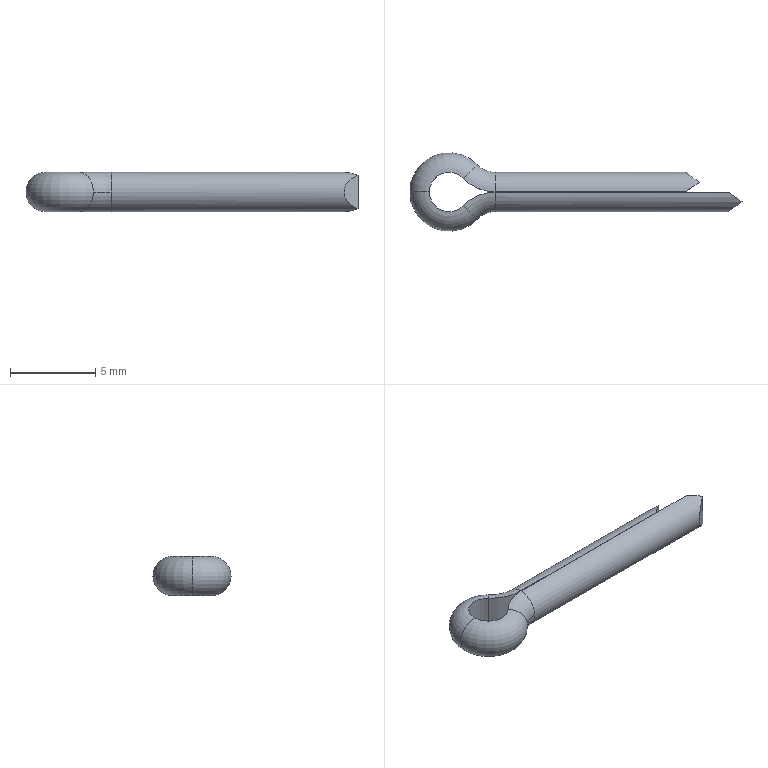Part | SolidWorks | features ICE 1, Sweep 1 | 1 solid | 17 faces | box 19.5 x 4.6 x 2.3 mm | volume 75.866 mm3 | torus 6 | plane 6 | cylinder 5 | commonest cylinder face diameters 2.3 x2 5.169 x2 2.32 x1
STEP:
#1=CARTESIAN_POINT('',(2.7,0.01,1.15));
#2=VERTEX_POINT('',#1);
#3=CARTESIAN_POINT('',(2.7,1.15,0.));
#4=VERTEX_POINT('',#3);
#5=CARTESIAN_POINT('',(2.7,0.,0.));
#6=DIRECTION('',(-1.,0.,0.));
#7=DIRECTION('',(0.,0.,1.));
#8=AXIS2_PLACEMENT_3D('',#5,#6,#7);
#9=CIRCLE('',#8,1.15);
#10=EDGE_CURVE('',#2,#4,#9,.T.);
#11=ORIENTED_EDGE('',*,*,#10,.T.);
#12=CARTESIAN_POINT('',(1.658,1.594,0.));
#13=VERTEX_POINT('',#12);
#14=CARTESIAN_POINT('',(2.7,2.595,0.));
#15=DIRECTION('',(0.,0.,-1.));
#16=DIRECTION('',(-1.,0.,0.));
#17=AXIS2_PLACEMENT_3D('',#14,#15,#16);
#18=CIRCLE('',#17,1.445);
#19=EDGE_CURVE('',#4,#13,#18,.T.);
#20=ORIENTED_EDGE('',*,*,#19,.T.);
#21=CARTESIAN_POINT('',(0.8364,0.8038,1.15));
#22=VERTEX_POINT('',#21);
#23=CARTESIAN_POINT('',(0.8292,0.7968,0.));
#24=DIRECTION('',(-0.6929,0.721,0.));
#25=DIRECTION('',(0.,0.,1.));
#26=AXIS2_PLACEMENT_3D('',#23,#24,#25);
#27=CIRCLE('',#26,1.15);
#28=EDGE_CURVE('',#22,#13,#27,.T.);
#29=ORIENTED_EDGE('',*,*,#28,.F.);
#30=CARTESIAN_POINT('',(2.7,2.595,1.15));
#31=DIRECTION('',(0.,0.,-1.));
#32=DIRECTION('',(-1.,0.,0.));
#33=AXIS2_PLACEMENT_3D('',#30,#31,#32);
#34=CIRCLE('',#33,2.585);
#35=EDGE_CURVE('',#2,#22,#34,.T.);
#36=ORIENTED_EDGE('',*,*,#35,.F.);
#37=EDGE_LOOP('',(#11,#20,#29,#36));
#38=FACE_OUTER_BOUND('',#37,.T.);
#39=CARTESIAN_POINT('',(2.7,2.595,0.));
#40=DIRECTION('',(0.,0.,-1.));
#41=DIRECTION('',(-1.,0.,0.));
#42=AXIS2_PLACEMENT_3D('',#39,#40,#41);
#43=TOROIDAL_SURFACE('',#42,2.595,1.15);
#44=ADVANCED_FACE('',(#38),#43,.T.);
#45=CARTESIAN_POINT('',(0.8364,-0.8038,1.15));
#46=VERTEX_POINT('',#45);
#47=CARTESIAN_POINT('',(1.658,-1.594,0.));
#48=VERTEX_POINT('',#47);
#49=CARTESIAN_POINT('',(0.8292,-0.7968,0.));
#50=DIRECTION('',(0.6929,0.721,0.));
#51=DIRECTION('',(0.,0.,1.));
#52=AXIS2_PLACEMENT_3D('',#49,#50,#51);
#53=CIRCLE('',#52,1.15);
#54=EDGE_CURVE('',#46,#48,#53,.T.);
#55=ORIENTED_EDGE('',*,*,#54,.T.);
#56=CARTESIAN_POINT('',(2.7,-1.15,0.));
#57=VERTEX_POINT('',#56);
#58=CARTESIAN_POINT('',(2.7,-2.595,0.));
#59=DIRECTION('',(0.,0.,-1.));
#60=DIRECTION('',(-1.,0.,0.));
#61=AXIS2_PLACEMENT_3D('',#58,#59,#60);
#62=CIRCLE('',#61,1.445);
#63=EDGE_CURVE('',#48,#57,#62,.T.);
#64=ORIENTED_EDGE('',*,*,#63,.T.);
#65=CARTESIAN_POINT('',(2.7,-0.01,1.15));
#66=VERTEX_POINT('',#65);
#67=CARTESIAN_POINT('',(2.7,0.,0.));
#68=DIRECTION('',(1.,0.,0.));
#69=DIRECTION('',(0.,0.,1.));
#70=AXIS2_PLACEMENT_3D('',#67,#68,#69);
#71=CIRCLE('',#70,1.15);
#72=EDGE_CURVE('',#66,#57,#71,.T.);
#73=ORIENTED_EDGE('',*,*,#72,.F.);
#74=CARTESIAN_POINT('',(2.7,-2.595,1.15));
#75=DIRECTION('',(0.,0.,-1.));
#76=DIRECTION('',(-1.,0.,0.));
#77=AXIS2_PLACEMENT_3D('',#74,#75,#76);
#78=CIRCLE('',#77,2.585);
#79=EDGE_CURVE('',#46,#66,#78,.T.);
#80=ORIENTED_EDGE('',*,*,#79,.F.);
#81=EDGE_LOOP('',(#55,#64,#73,#80));
#82=FACE_OUTER_BOUND('',#81,.T.);
#83=CARTESIAN_POINT('',(2.7,-2.595,0.));
#84=DIRECTION('',(0.,0.,-1.));
#85=DIRECTION('',(-1.,0.,0.));
#86=AXIS2_PLACEMENT_3D('',#83,#84,#85);
#87=TOROIDAL_SURFACE('',#86,2.595,1.15);
#88=ADVANCED_FACE('',(#82),#87,.T.);
#89=CARTESIAN_POINT('',(0.8364,0.8038,-1.15));
#90=VERTEX_POINT('',#89);
#91=CARTESIAN_POINT('',(-1.16,0.,-1.15));
#92=VERTEX_POINT('',#91);
#93=CARTESIAN_POINT('',(0.,0.,-1.15));
#94=DIRECTION('',(0.,0.,1.));
#95=DIRECTION('',(1.,0.,0.));
#96=AXIS2_PLACEMENT_3D('',#93,#94,#95);
#97=CIRCLE('',#96,1.16);
#98=EDGE_CURVE('',#90,#92,#97,.T.);
#99=ORIENTED_EDGE('',*,*,#98,.T.);
#100=CARTESIAN_POINT('',(-1.16,0.,1.15));
#101=VERTEX_POINT('',#100);
#102=CARTESIAN_POINT('',(-1.15,0.,0.));
#103=DIRECTION('',(0.,1.,0.));
#104=DIRECTION('',(-1.,0.,0.));
#105=AXIS2_PLACEMENT_3D('',#102,#103,#104);
#106=CIRCLE('',#105,1.15);
#107=EDGE_CURVE('',#92,#101,#106,.T.);
#108=ORIENTED_EDGE('',*,*,#107,.T.);
#109=CARTESIAN_POINT('',(0.,0.,1.15));
#110=DIRECTION('',(0.,0.,1.));
#111=DIRECTION('',(1.,0.,0.));
#112=AXIS2_PLACEMENT_3D('',#109,#110,#111);
#113=CIRCLE('',#112,1.16);
#114=EDGE_CURVE('',#22,#101,#113,.T.);
#115=ORIENTED_EDGE('',*,*,#114,.F.);
#116=ORIENTED_EDGE('',*,*,#28,.T.);
#117=CARTESIAN_POINT('',(0.8292,0.7968,0.));
#118=DIRECTION('',(-0.6929,0.721,0.));
#119=DIRECTION('',(0.,0.,1.));
#120=AXIS2_PLACEMENT_3D('',#117,#118,#119);
#121=CIRCLE('',#120,1.15);
#122=EDGE_CURVE('',#13,#90,#121,.T.);
#123=ORIENTED_EDGE('',*,*,#122,.T.);
#124=EDGE_LOOP('',(#99,#108,#115,#116,#123));
#125=FACE_OUTER_BOUND('',#124,.T.);
#126=CARTESIAN_POINT('',(0.,0.,0.));
#127=DIRECTION('',(0.,0.,1.));
#128=DIRECTION('',(1.,0.,0.));
#129=AXIS2_PLACEMENT_3D('',#126,#127,#128);
#130=TOROIDAL_SURFACE('',#129,1.15,1.15);
#131=ADVANCED_FACE('',(#125),#130,.T.);
#132=CARTESIAN_POINT('',(17.2,-0.58,-0.993));
#133=VERTEX_POINT('',#132);
#134=CARTESIAN_POINT('',(16.396,-0.01,-1.15));
#135=VERTEX_POINT('',#134);
#136=CARTESIAN_POINT('',(17.2,-0.58,-0.993));
#137=CARTESIAN_POINT('',(16.955,-0.4059,-1.095));
#138=CARTESIAN_POINT('',(16.681,-0.2116,-1.148));
#139=CARTESIAN_POINT('',(16.396,-0.01,-1.15));
#140=(BOUNDED_CURVE()B_SPLINE_CURVE(3,(#136,#137,#138,#139),.UNSPECIFIED.,.F.,.F.)B_SPLINE_CURVE_WITH_KNOTS((4,4),(1.042,1.562),.UNSPECIFIED.)CURVE()GEOMETRIC_REPRESENTATION_ITEM()RATIONAL_B_SPLINE_CURVE((1.,0.9776,0.9776,1.))REPRESENTATION_ITEM(''));
#141=EDGE_CURVE('',#133,#135,#140,.T.);
#142=ORIENTED_EDGE('',*,*,#141,.F.);
#143=CARTESIAN_POINT('',(17.2,-0.58,0.993));
#144=VERTEX_POINT('',#143);
#145=CARTESIAN_POINT('',(17.2,-0.58,0.993));
#146=CARTESIAN_POINT('',(15.965,-1.434,0.4944));
#147=CARTESIAN_POINT('',(15.965,-1.434,-0.4944));
#148=CARTESIAN_POINT('',(17.2,-0.58,-0.993));
#149=(BOUNDED_CURVE()B_SPLINE_CURVE(3,(#145,#146,#147,#148),.UNSPECIFIED.,.F.,.F.)B_SPLINE_CURVE_WITH_KNOTS((4,4),(2.099,4.184),.UNSPECIFIED.)CURVE()GEOMETRIC_REPRESENTATION_ITEM()RATIONAL_B_SPLINE_CURVE((1.,0.6696,0.6696,1.))REPRESENTATION_ITEM(''));
#150=EDGE_CURVE('',#144,#133,#149,.T.);
#151=ORIENTED_EDGE('',*,*,#150,.F.);
#152=CARTESIAN_POINT('',(16.396,-0.01,1.15));
#153=VERTEX_POINT('',#152);
#154=CARTESIAN_POINT('',(16.396,-0.01,1.15));
#155=CARTESIAN_POINT('',(16.681,-0.2116,1.148));
#156=CARTESIAN_POINT('',(16.955,-0.4059,1.095));
#157=CARTESIAN_POINT('',(17.2,-0.58,0.993));
#158=(BOUNDED_CURVE()B_SPLINE_CURVE(3,(#154,#155,#156,#157),.UNSPECIFIED.,.F.,.F.)B_SPLINE_CURVE_WITH_KNOTS((4,4),(4.721,5.241),.UNSPECIFIED.)CURVE()GEOMETRIC_REPRESENTATION_ITEM()RATIONAL_B_SPLINE_CURVE((1.,0.9776,0.9776,1.))REPRESENTATION_ITEM(''));
#159=EDGE_CURVE('',#153,#144,#158,.T.);
#160=ORIENTED_EDGE('',*,*,#159,.F.);
#161=CARTESIAN_POINT('',(2.7,-0.01,1.15));
#162=DIRECTION('',(1.,0.,0.));
#163=VECTOR('',#162,1000.);
#164=LINE('',#161,#163);
#165=EDGE_CURVE('',#66,#153,#164,.T.);
#166=ORIENTED_EDGE('',*,*,#165,.F.);
#167=ORIENTED_EDGE('',*,*,#72,.T.);
#168=CARTESIAN_POINT('',(2.7,-0.01,-1.15));
#169=VERTEX_POINT('',#168);
#170=CARTESIAN_POINT('',(2.7,0.,0.));
#171=DIRECTION('',(1.,0.,0.));
#172=DIRECTION('',(0.,0.,1.));
#173=AXIS2_PLACEMENT_3D('',#170,#171,#172);
#174=CIRCLE('',#173,1.15);
#175=EDGE_CURVE('',#57,#169,#174,.T.);
#176=ORIENTED_EDGE('',*,*,#175,.T.);
#177=CARTESIAN_POINT('',(2.7,-0.01,-1.15));
#178=DIRECTION('',(1.,0.,0.));
#179=VECTOR('',#178,1000.);
#180=LINE('',#177,#179);
#181=EDGE_CURVE('',#169,#135,#180,.T.);
#182=ORIENTED_EDGE('',*,*,#181,.T.);
#183=EDGE_LOOP('',(#142,#151,#160,#166,#167,#176,#182));
#184=FACE_OUTER_BOUND('',#183,.T.);
#185=CARTESIAN_POINT('',(2.7,0.,0.));
#186=DIRECTION('',(1.,0.,0.));
#187=DIRECTION('',(0.,1.,0.));
#188=AXIS2_PLACEMENT_3D('',#185,#186,#187);
#189=CYLINDRICAL_SURFACE('',#188,1.15);
#190=ADVANCED_FACE('',(#184),#189,.T.);
#191=CARTESIAN_POINT('',(16.396,-0.01,-1.15));
#192=DIRECTION('',(0.,0.,1.));
#193=VECTOR('',#192,1000.);
#194=LINE('',#191,#193);
#195=EDGE_CURVE('',#135,#153,#194,.T.);
#196=ORIENTED_EDGE('',*,*,#195,.F.);
#197=ORIENTED_EDGE('',*,*,#181,.F.);
#198=CARTESIAN_POINT('',(2.7,-0.01,-1.15));
#199=DIRECTION('',(0.,0.,1.));
#200=VECTOR('',#199,1000.);
#201=LINE('',#198,#200);
#202=EDGE_CURVE('',#169,#66,#201,.T.);
#203=ORIENTED_EDGE('',*,*,#202,.T.);
#204=ORIENTED_EDGE('',*,*,#165,.T.);
#205=EDGE_LOOP('',(#196,#197,#203,#204));
#206=FACE_OUTER_BOUND('',#205,.T.);
#207=CARTESIAN_POINT('',(2.7,-0.01,-1.15));
#208=DIRECTION('',(0.,1.,0.));
#209=DIRECTION('',(-1.,0.,0.));
#210=AXIS2_PLACEMENT_3D('',#207,#208,#209);
#211=PLANE('',#210);
#212=ADVANCED_FACE('',(#206),#211,.T.);
#213=CARTESIAN_POINT('',(0.8364,-0.8038,-1.15));
#214=VERTEX_POINT('',#213);
#215=CARTESIAN_POINT('',(0.8364,-0.8038,-1.15));
#216=DIRECTION('',(0.,0.,1.));
#217=VECTOR('',#216,1000.);
#218=LINE('',#215,#217);
#219=EDGE_CURVE('',#214,#46,#218,.T.);
#220=ORIENTED_EDGE('',*,*,#219,.T.);
#221=ORIENTED_EDGE('',*,*,#79,.T.);
#222=ORIENTED_EDGE('',*,*,#202,.F.);
#223=CARTESIAN_POINT('',(2.7,-2.595,-1.15));
#224=DIRECTION('',(0.,0.,-1.));
#225=DIRECTION('',(-1.,0.,0.));
#226=AXIS2_PLACEMENT_3D('',#223,#224,#225);
#227=CIRCLE('',#226,2.585);
#228=EDGE_CURVE('',#214,#169,#227,.T.);
#229=ORIENTED_EDGE('',*,*,#228,.F.);
#230=EDGE_LOOP('',(#220,#221,#222,#229));
#231=FACE_OUTER_BOUND('',#230,.T.);
#232=CARTESIAN_POINT('',(2.7,-2.595,0.));
#233=DIRECTION('',(0.,0.,-1.));
#234=DIRECTION('',(-1.,0.,0.));
#235=AXIS2_PLACEMENT_3D('',#232,#233,#234);
#236=CYLINDRICAL_SURFACE('',#235,2.585);
#237=ADVANCED_FACE('',(#231),#236,.T.);
#238=ORIENTED_EDGE('',*,*,#63,.F.);
#239=CARTESIAN_POINT('',(0.8292,-0.7968,0.));
#240=DIRECTION('',(0.6929,0.721,0.));
#241=DIRECTION('',(0.,0.,1.));
#242=AXIS2_PLACEMENT_3D('',#239,#240,#241);
#243=CIRCLE('',#242,1.15);
#244=EDGE_CURVE('',#48,#214,#243,.T.);
#245=ORIENTED_EDGE('',*,*,#244,.T.);
#246=ORIENTED_EDGE('',*,*,#228,.T.);
#247=ORIENTED_EDGE('',*,*,#175,.F.);
#248=EDGE_LOOP('',(#238,#245,#246,#247));
#249=FACE_OUTER_BOUND('',#248,.T.);
#250=CARTESIAN_POINT('',(2.7,-2.595,0.));
#251=DIRECTION('',(0.,0.,-1.));
#252=DIRECTION('',(-1.,0.,0.));
#253=AXIS2_PLACEMENT_3D('',#250,#251,#252);
#254=TOROIDAL_SURFACE('',#253,2.595,1.15);
#255=ADVANCED_FACE('',(#249),#254,.T.);
#256=CARTESIAN_POINT('',(0.8364,0.8038,-1.15));
#257=DIRECTION('',(0.,0.,1.));
#258=VECTOR('',#257,1000.);
#259=LINE('',#256,#258);
#260=EDGE_CURVE('',#90,#22,#259,.T.);
#261=ORIENTED_EDGE('',*,*,#260,.T.);
#262=ORIENTED_EDGE('',*,*,#114,.T.);
#263=CARTESIAN_POINT('',(0.,0.,1.15));
#264=DIRECTION('',(0.,0.,1.));
#265=DIRECTION('',(1.,0.,0.));
#266=AXIS2_PLACEMENT_3D('',#263,#264,#265);
#267=CIRCLE('',#266,1.16);
#268=EDGE_CURVE('',#101,#46,#267,.T.);
#269=ORIENTED_EDGE('',*,*,#268,.T.);
#270=ORIENTED_EDGE('',*,*,#219,.F.);
#271=CARTESIAN_POINT('',(0.,0.,-1.15));
#272=DIRECTION('',(0.,0.,1.));
#273=DIRECTION('',(1.,0.,0.));
#274=AXIS2_PLACEMENT_3D('',#271,#272,#273);
#275=CIRCLE('',#274,1.16);
#276=EDGE_CURVE('',#92,#214,#275,.T.);
#277=ORIENTED_EDGE('',*,*,#276,.F.);
#278=ORIENTED_EDGE('',*,*,#98,.F.);
#279=EDGE_LOOP('',(#261,#262,#269,#270,#277,#278));
#280=FACE_OUTER_BOUND('',#279,.T.);
#281=CARTESIAN_POINT('',(0.,0.,0.));
#282=DIRECTION('',(0.,0.,1.));
#283=DIRECTION('',(1.,0.,0.));
#284=AXIS2_PLACEMENT_3D('',#281,#282,#283);
#285=CYLINDRICAL_SURFACE('',#284,1.16);
#286=ADVANCED_FACE('',(#280),#285,.F.);
#287=ORIENTED_EDGE('',*,*,#107,.F.);
#288=ORIENTED_EDGE('',*,*,#276,.T.);
#289=ORIENTED_EDGE('',*,*,#244,.F.);
#290=ORIENTED_EDGE('',*,*,#54,.F.);
#291=ORIENTED_EDGE('',*,*,#268,.F.);
#292=EDGE_LOOP('',(#287,#288,#289,#290,#291));
#293=FACE_OUTER_BOUND('',#292,.T.);
#294=CARTESIAN_POINT('',(0.,0.,0.));
#295=DIRECTION('',(0.,0.,1.));
#296=DIRECTION('',(1.,0.,0.));
#297=AXIS2_PLACEMENT_3D('',#294,#295,#296);
#298=TOROIDAL_SURFACE('',#297,1.15,1.15);
#299=ADVANCED_FACE('',(#293),#298,.T.);
#300=CARTESIAN_POINT('',(2.7,0.01,-1.15));
#301=VERTEX_POINT('',#300);
#302=CARTESIAN_POINT('',(2.7,0.01,-1.15));
#303=DIRECTION('',(0.,0.,1.));
#304=VECTOR('',#303,1000.);
#305=LINE('',#302,#304);
#306=EDGE_CURVE('',#301,#2,#305,.T.);
#307=ORIENTED_EDGE('',*,*,#306,.T.);
#308=ORIENTED_EDGE('',*,*,#35,.T.);
#309=ORIENTED_EDGE('',*,*,#260,.F.);
#310=CARTESIAN_POINT('',(2.7,2.595,-1.15));
#311=DIRECTION('',(0.,0.,-1.));
#312=DIRECTION('',(-1.,0.,0.));
#313=AXIS2_PLACEMENT_3D('',#310,#311,#312);
#314=CIRCLE('',#313,2.585);
#315=EDGE_CURVE('',#301,#90,#314,.T.);
#316=ORIENTED_EDGE('',*,*,#315,.F.);
#317=EDGE_LOOP('',(#307,#308,#309,#316));
#318=FACE_OUTER_BOUND('',#317,.T.);
#319=CARTESIAN_POINT('',(2.7,2.595,0.));
#320=DIRECTION('',(0.,0.,-1.));
#321=DIRECTION('',(-1.,0.,0.));
#322=AXIS2_PLACEMENT_3D('',#319,#320,#321);
#323=CYLINDRICAL_SURFACE('',#322,2.585);
#324=ADVANCED_FACE('',(#318),#323,.T.);
#325=ORIENTED_EDGE('',*,*,#19,.F.);
#326=CARTESIAN_POINT('',(2.7,0.,0.));
#327=DIRECTION('',(-1.,0.,0.));
#328=DIRECTION('',(0.,0.,1.));
#329=AXIS2_PLACEMENT_3D('',#326,#327,#328);
#330=CIRCLE('',#329,1.15);
#331=EDGE_CURVE('',#4,#301,#330,.T.);
#332=ORIENTED_EDGE('',*,*,#331,.T.);
#333=ORIENTED_EDGE('',*,*,#315,.T.);
#334=ORIENTED_EDGE('',*,*,#122,.F.);
#335=EDGE_LOOP('',(#325,#332,#333,#334));
#336=FACE_OUTER_BOUND('',#335,.T.);
#337=CARTESIAN_POINT('',(2.7,2.595,0.));
#338=DIRECTION('',(0.,0.,-1.));
#339=DIRECTION('',(-1.,0.,0.));
#340=AXIS2_PLACEMENT_3D('',#337,#338,#339);
#341=TOROIDAL_SURFACE('',#340,2.595,1.15);
#342=ADVANCED_FACE('',(#336),#341,.T.);
#343=CARTESIAN_POINT('',(13.89,0.01,1.15));
#344=VERTEX_POINT('',#343);
#345=CARTESIAN_POINT('',(2.7,0.01,1.15));
#346=DIRECTION('',(1.,0.,0.));
#347=VECTOR('',#346,1000.);
#348=LINE('',#345,#347);
#349=EDGE_CURVE('',#2,#344,#348,.T.);
#350=ORIENTED_EDGE('',*,*,#349,.T.);
#351=CARTESIAN_POINT('',(14.7,0.57,0.9988));
#352=VERTEX_POINT('',#351);
#353=CARTESIAN_POINT('',(13.89,0.01,1.15));
#354=CARTESIAN_POINT('',(14.176,0.2076,1.148));
#355=CARTESIAN_POINT('',(14.452,0.3984,1.097));
#356=CARTESIAN_POINT('',(14.7,0.57,0.9988));
#357=(BOUNDED_CURVE()B_SPLINE_CURVE(3,(#353,#354,#355,#356),.UNSPECIFIED.,.F.,.F.)B_SPLINE_CURVE_WITH_KNOTS((4,4),(4.721,5.231),.UNSPECIFIED.)CURVE()GEOMETRIC_REPRESENTATION_ITEM()RATIONAL_B_SPLINE_CURVE((1.,0.9785,0.9785,1.))REPRESENTATION_ITEM(''));
#358=EDGE_CURVE('',#344,#352,#357,.T.);
#359=ORIENTED_EDGE('',*,*,#358,.T.);
#360=CARTESIAN_POINT('',(14.7,0.57,-0.9988));
#361=VERTEX_POINT('',#360);
#362=CARTESIAN_POINT('',(14.7,0.57,0.9988));
#363=CARTESIAN_POINT('',(13.472,1.441,0.5016));
#364=CARTESIAN_POINT('',(13.472,1.441,-0.5016));
#365=CARTESIAN_POINT('',(14.7,0.57,-0.9988));
#366=(BOUNDED_CURVE()B_SPLINE_CURVE(3,(#362,#363,#364,#365),.UNSPECIFIED.,.F.,.F.)B_SPLINE_CURVE_WITH_KNOTS((4,4),(2.089,4.194),.UNSPECIFIED.)CURVE()GEOMETRIC_REPRESENTATION_ITEM()RATIONAL_B_SPLINE_CURVE((1.,0.6638,0.6638,1.))REPRESENTATION_ITEM(''));
#367=EDGE_CURVE('',#352,#361,#366,.T.);
#368=ORIENTED_EDGE('',*,*,#367,.T.);
#369=CARTESIAN_POINT('',(13.89,0.01,-1.15));
#370=VERTEX_POINT('',#369);
#371=CARTESIAN_POINT('',(14.7,0.57,-0.9988));
#372=CARTESIAN_POINT('',(14.452,0.3984,-1.097));
#373=CARTESIAN_POINT('',(14.176,0.2076,-1.148));
#374=CARTESIAN_POINT('',(13.89,0.01,-1.15));
#375=(BOUNDED_CURVE()B_SPLINE_CURVE(3,(#371,#372,#373,#374),.UNSPECIFIED.,.F.,.F.)B_SPLINE_CURVE_WITH_KNOTS((4,4),(1.052,1.562),.UNSPECIFIED.)CURVE()GEOMETRIC_REPRESENTATION_ITEM()RATIONAL_B_SPLINE_CURVE((1.,0.9785,0.9785,1.))REPRESENTATION_ITEM(''));
#376=EDGE_CURVE('',#361,#370,#375,.T.);
#377=ORIENTED_EDGE('',*,*,#376,.T.);
#378=CARTESIAN_POINT('',(2.7,0.01,-1.15));
#379=DIRECTION('',(1.,0.,0.));
#380=VECTOR('',#379,1000.);
#381=LINE('',#378,#380);
#382=EDGE_CURVE('',#301,#370,#381,.T.);
#383=ORIENTED_EDGE('',*,*,#382,.F.);
#384=ORIENTED_EDGE('',*,*,#331,.F.);
#385=ORIENTED_EDGE('',*,*,#10,.F.);
#386=EDGE_LOOP('',(#350,#359,#368,#377,#383,#384,#385));
#387=FACE_OUTER_BOUND('',#386,.T.);
#388=CARTESIAN_POINT('',(2.7,0.,0.));
#389=DIRECTION('',(1.,0.,0.));
#390=DIRECTION('',(0.,0.,-1.));
#391=AXIS2_PLACEMENT_3D('',#388,#389,#390);
#392=CYLINDRICAL_SURFACE('',#391,1.15);
#393=ADVANCED_FACE('',(#387),#392,.T.);
#394=ORIENTED_EDGE('',*,*,#382,.T.);
#395=CARTESIAN_POINT('',(13.89,0.01,-1.15));
#396=DIRECTION('',(0.,0.,1.));
#397=VECTOR('',#396,1000.);
#398=LINE('',#395,#397);
#399=EDGE_CURVE('',#370,#344,#398,.T.);
#400=ORIENTED_EDGE('',*,*,#399,.T.);
#401=ORIENTED_EDGE('',*,*,#349,.F.);
#402=ORIENTED_EDGE('',*,*,#306,.F.);
#403=EDGE_LOOP('',(#394,#400,#401,#402));
#404=FACE_OUTER_BOUND('',#403,.T.);
#405=CARTESIAN_POINT('',(2.7,0.01,-1.15));
#406=DIRECTION('',(0.,1.,0.));
#407=DIRECTION('',(0.,0.,1.));
#408=AXIS2_PLACEMENT_3D('',#405,#406,#407);
#409=PLANE('',#408);
#410=ADVANCED_FACE('',(#404),#409,.F.);
#411=CARTESIAN_POINT('',(14.7,0.57,-1.15));
#412=DIRECTION('',(0.,0.,1.));
#413=VECTOR('',#412,1000.);
#414=LINE('',#411,#413);
#415=EDGE_CURVE('',#361,#352,#414,.T.);
#416=ORIENTED_EDGE('',*,*,#415,.T.);
#417=ORIENTED_EDGE('',*,*,#358,.F.);
#418=ORIENTED_EDGE('',*,*,#399,.F.);
#419=ORIENTED_EDGE('',*,*,#376,.F.);
#420=EDGE_LOOP('',(#416,#417,#418,#419));
#421=FACE_OUTER_BOUND('',#420,.T.);
#422=CARTESIAN_POINT('',(14.7,0.57,-1.15));
#423=DIRECTION('',(-0.5686,0.8226,0.));
#424=DIRECTION('',(-0.8226,-0.5686,0.));
#425=AXIS2_PLACEMENT_3D('',#422,#423,#424);
#426=PLANE('',#425);
#427=ADVANCED_FACE('',(#421),#426,.F.);
#428=ORIENTED_EDGE('',*,*,#415,.F.);
#429=ORIENTED_EDGE('',*,*,#367,.F.);
#430=EDGE_LOOP('',(#428,#429));
#431=FACE_OUTER_BOUND('',#430,.T.);
#432=CARTESIAN_POINT('',(14.7,0.57,-1.15));
#433=DIRECTION('',(-0.5786,-0.8156,0.));
#434=DIRECTION('',(0.8156,-0.5786,0.));
#435=AXIS2_PLACEMENT_3D('',#432,#433,#434);
#436=PLANE('',#435);
#437=ADVANCED_FACE('',(#431),#436,.F.);
#438=ORIENTED_EDGE('',*,*,#150,.T.);
#439=CARTESIAN_POINT('',(17.2,-0.58,-1.15));
#440=DIRECTION('',(0.,0.,1.));
#441=VECTOR('',#440,1000.);
#442=LINE('',#439,#441);
#443=EDGE_CURVE('',#133,#144,#442,.T.);
#444=ORIENTED_EDGE('',*,*,#443,.T.);
#445=EDGE_LOOP('',(#438,#444));
#446=FACE_OUTER_BOUND('',#445,.T.);
#447=CARTESIAN_POINT('',(17.2,-0.58,-1.15));
#448=DIRECTION('',(-0.5686,0.8226,0.));
#449=DIRECTION('',(-0.8226,-0.5686,0.));
#450=AXIS2_PLACEMENT_3D('',#447,#448,#449);
#451=PLANE('',#450);
#452=ADVANCED_FACE('',(#446),#451,.F.);
#453=ORIENTED_EDGE('',*,*,#141,.T.);
#454=ORIENTED_EDGE('',*,*,#195,.T.);
#455=ORIENTED_EDGE('',*,*,#159,.T.);
#456=ORIENTED_EDGE('',*,*,#443,.F.);
#457=EDGE_LOOP('',(#453,#454,#455,#456));
#458=FACE_OUTER_BOUND('',#457,.T.);
#459=CARTESIAN_POINT('',(17.2,-0.58,-1.15));
#460=DIRECTION('',(-0.5786,-0.8156,0.));
#461=DIRECTION('',(0.8156,-0.5786,0.));
#462=AXIS2_PLACEMENT_3D('',#459,#460,#461);
#463=PLANE('',#462);
#464=ADVANCED_FACE('',(#458),#463,.F.);
#465=CLOSED_SHELL('',(#44,#88,#131,#190,#212,#237,#255,#286,#299,#324,#342,#393,#410,#427,#437,#452,#464));
#466=MANIFOLD_SOLID_BREP('',#465);
#467=CARTESIAN_POINT('',(0.,0.,0.));
#468=DIRECTION('',(0.,0.,1.));
#469=DIRECTION('',(1.,0.,0.));
#470=AXIS2_PLACEMENT_3D('',#467,#468,#469);
#471=(LENGTH_UNIT()NAMED_UNIT(*)SI_UNIT(.MILLI.,.METRE.));
#472=UNCERTAINTY_MEASURE_WITH_UNIT(LENGTH_MEASURE(0.00001),#471,'','');
#473=(NAMED_UNIT(*)PLANE_ANGLE_UNIT()SI_UNIT($,.RADIAN.));
#474=(NAMED_UNIT(*)SI_UNIT($,.STERADIAN.)SOLID_ANGLE_UNIT());
#475=(GEOMETRIC_REPRESENTATION_CONTEXT(3)GLOBAL_UNCERTAINTY_ASSIGNED_CONTEXT((#472))GLOBAL_UNIT_ASSIGNED_CONTEXT((#471,#473,#474))REPRESENTATION_CONTEXT('',''));
#476=ADVANCED_BREP_SHAPE_REPRESENTATION('',(#466,#470),#475);